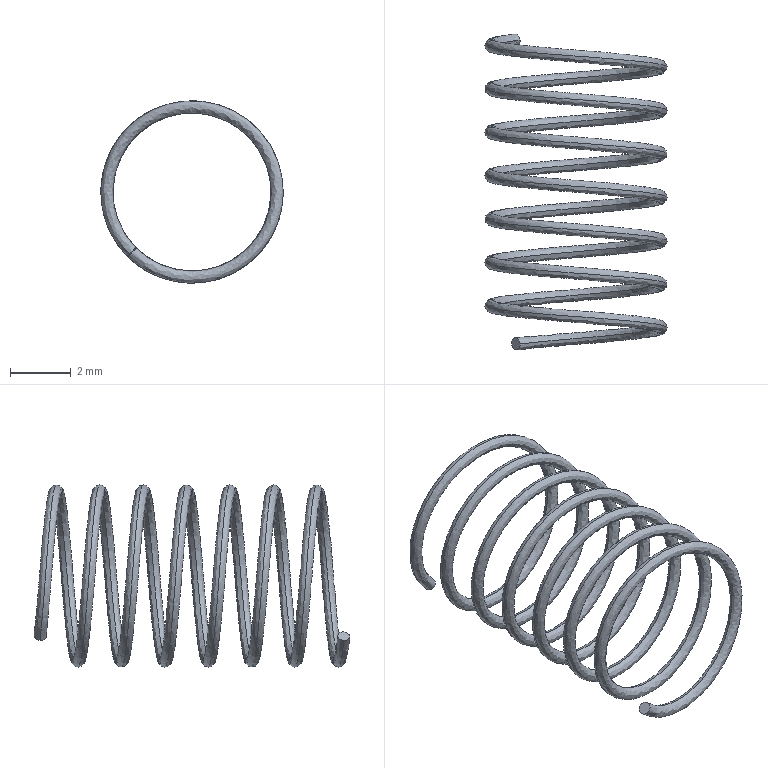Part | SolidWorks | features Helix 1, RefAxis 1, Sweep 1 | 1 solid | 4 faces | box 6 x 10.399 x 6 mm | volume 15.53 mm3 | spline 2 | plane 2